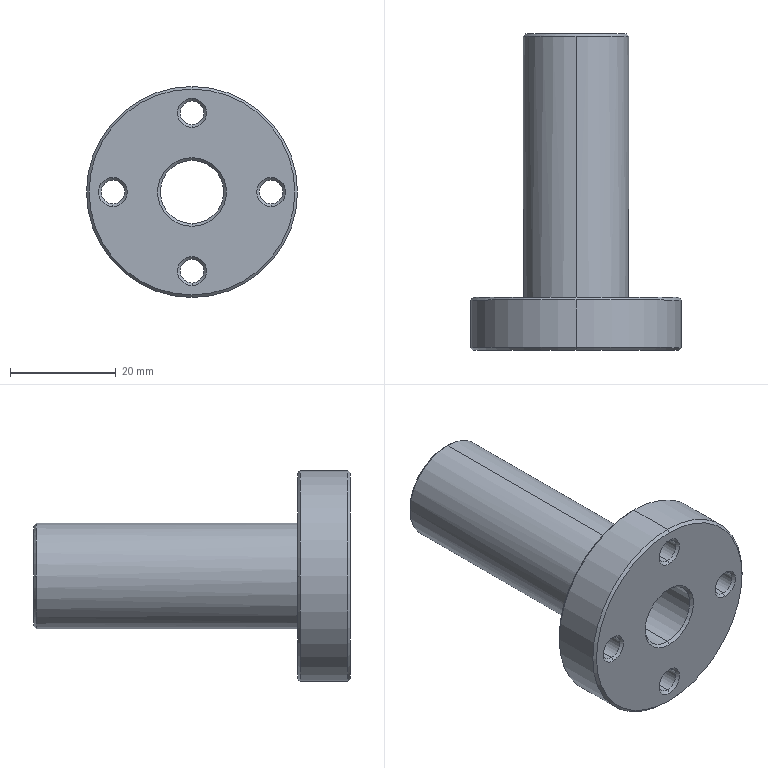Part | STEP file | 04-02 Suction guide sleeve | 1 solid | 43 faces | box 40 x 60 x 40 mm | volume 20789 mm3 | cone 26 | cylinder 14 | plane 3 | commonest cylinder face diameters 4.5 x8 12 x2 20 x2 40 x2